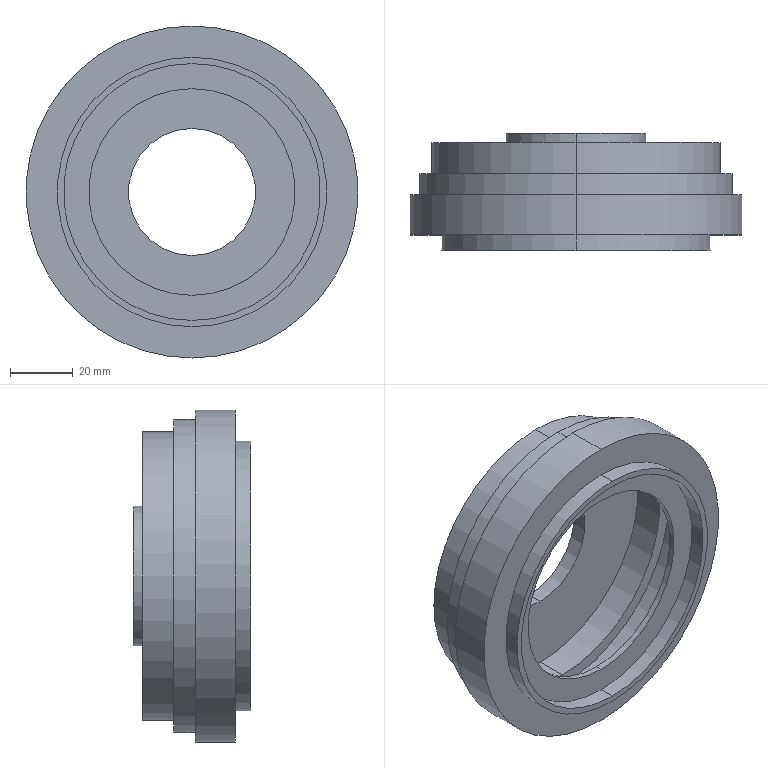Part | SolidWorks | features Revolution 1 | 1 solid | 33 faces | box 106 x 37.5 x 106 mm | volume 44844 mm3 | cylinder 22 | plane 11 | commonest cylinder face diameters 40.568 x2 44.568 x2 66 x2 82 x2 86 x2 88 x2
STEP:
#1=CARTESIAN_POINT('',(0.,136.,43.));
#2=VERTEX_POINT('',#1);
#3=CARTESIAN_POINT('',(0.,136.,-43.));
#4=VERTEX_POINT('',#3);
#5=CARTESIAN_POINT('',(0.,136.,0.));
#6=DIRECTION('',(0.,1.,0.));
#7=DIRECTION('',(0.,0.,1.));
#8=AXIS2_PLACEMENT_3D('',#5,#6,#7);
#9=CIRCLE('',#8,43.);
#10=EDGE_CURVE('',#2,#4,#9,.T.);
#11=ORIENTED_EDGE('',*,*,#10,.T.);
#12=CARTESIAN_POINT('',(0.,141.,-43.));
#13=VERTEX_POINT('',#12);
#14=CARTESIAN_POINT('',(0.,0.,-43.));
#15=DIRECTION('',(0.,1.,0.));
#16=VECTOR('',#15,1000.);
#17=LINE('',#14,#16);
#18=EDGE_CURVE('',#4,#13,#17,.T.);
#19=ORIENTED_EDGE('',*,*,#18,.T.);
#20=CARTESIAN_POINT('',(0.,141.,43.));
#21=VERTEX_POINT('',#20);
#22=CARTESIAN_POINT('',(0.,141.,0.));
#23=DIRECTION('',(0.,1.,0.));
#24=DIRECTION('',(0.,0.,1.));
#25=AXIS2_PLACEMENT_3D('',#22,#23,#24);
#26=CIRCLE('',#25,43.);
#27=EDGE_CURVE('',#21,#13,#26,.T.);
#28=ORIENTED_EDGE('',*,*,#27,.F.);
#29=CARTESIAN_POINT('',(0.,0.,43.));
#30=DIRECTION('',(0.,1.,0.));
#31=VECTOR('',#30,1000.);
#32=LINE('',#29,#31);
#33=EDGE_CURVE('',#2,#21,#32,.T.);
#34=ORIENTED_EDGE('',*,*,#33,.F.);
#35=EDGE_LOOP('',(#11,#19,#28,#34));
#36=FACE_OUTER_BOUND('',#35,.T.);
#37=CARTESIAN_POINT('',(0.,0.,0.));
#38=DIRECTION('',(0.,1.,0.));
#39=DIRECTION('',(0.,0.,1.));
#40=AXIS2_PLACEMENT_3D('',#37,#38,#39);
#41=CYLINDRICAL_SURFACE('',#40,43.);
#42=ADVANCED_FACE('',(#36),#41,.T.);
#43=CARTESIAN_POINT('',(0.,141.,53.));
#44=VERTEX_POINT('',#43);
#45=CARTESIAN_POINT('',(0.,141.,-53.));
#46=VERTEX_POINT('',#45);
#47=CARTESIAN_POINT('',(0.,141.,0.));
#48=DIRECTION('',(0.,1.,0.));
#49=DIRECTION('',(0.,0.,1.));
#50=AXIS2_PLACEMENT_3D('',#47,#48,#49);
#51=CIRCLE('',#50,53.);
#52=EDGE_CURVE('',#44,#46,#51,.T.);
#53=ORIENTED_EDGE('',*,*,#52,.T.);
#54=CARTESIAN_POINT('',(0.,153.773,-53.));
#55=VERTEX_POINT('',#54);
#56=CARTESIAN_POINT('',(0.,0.,-53.));
#57=DIRECTION('',(0.,1.,0.));
#58=VECTOR('',#57,1000.);
#59=LINE('',#56,#58);
#60=EDGE_CURVE('',#46,#55,#59,.T.);
#61=ORIENTED_EDGE('',*,*,#60,.T.);
#62=CARTESIAN_POINT('',(0.,153.773,53.));
#63=VERTEX_POINT('',#62);
#64=CARTESIAN_POINT('',(0.,153.773,0.));
#65=DIRECTION('',(0.,1.,0.));
#66=DIRECTION('',(0.,0.,1.));
#67=AXIS2_PLACEMENT_3D('',#64,#65,#66);
#68=CIRCLE('',#67,53.);
#69=EDGE_CURVE('',#63,#55,#68,.T.);
#70=ORIENTED_EDGE('',*,*,#69,.F.);
#71=CARTESIAN_POINT('',(0.,0.,53.));
#72=DIRECTION('',(0.,1.,0.));
#73=VECTOR('',#72,1000.);
#74=LINE('',#71,#73);
#75=EDGE_CURVE('',#44,#63,#74,.T.);
#76=ORIENTED_EDGE('',*,*,#75,.F.);
#77=EDGE_LOOP('',(#53,#61,#70,#76));
#78=FACE_OUTER_BOUND('',#77,.T.);
#79=CARTESIAN_POINT('',(0.,0.,0.));
#80=DIRECTION('',(0.,1.,0.));
#81=DIRECTION('',(0.,0.,1.));
#82=AXIS2_PLACEMENT_3D('',#79,#80,#81);
#83=CYLINDRICAL_SURFACE('',#82,53.);
#84=ADVANCED_FACE('',(#78),#83,.T.);
#85=CARTESIAN_POINT('',(0.,153.773,50.));
#86=VERTEX_POINT('',#85);
#87=CARTESIAN_POINT('',(0.,153.773,-50.));
#88=VERTEX_POINT('',#87);
#89=CARTESIAN_POINT('',(0.,153.773,0.));
#90=DIRECTION('',(0.,1.,0.));
#91=DIRECTION('',(0.,0.,1.));
#92=AXIS2_PLACEMENT_3D('',#89,#90,#91);
#93=CIRCLE('',#92,50.);
#94=EDGE_CURVE('',#86,#88,#93,.T.);
#95=ORIENTED_EDGE('',*,*,#94,.T.);
#96=CARTESIAN_POINT('',(0.,160.532,-50.));
#97=VERTEX_POINT('',#96);
#98=CARTESIAN_POINT('',(0.,0.,-50.));
#99=DIRECTION('',(0.,1.,0.));
#100=VECTOR('',#99,1000.);
#101=LINE('',#98,#100);
#102=EDGE_CURVE('',#88,#97,#101,.T.);
#103=ORIENTED_EDGE('',*,*,#102,.T.);
#104=CARTESIAN_POINT('',(0.,160.532,50.));
#105=VERTEX_POINT('',#104);
#106=CARTESIAN_POINT('',(0.,160.532,0.));
#107=DIRECTION('',(0.,1.,0.));
#108=DIRECTION('',(0.,0.,1.));
#109=AXIS2_PLACEMENT_3D('',#106,#107,#108);
#110=CIRCLE('',#109,50.);
#111=EDGE_CURVE('',#105,#97,#110,.T.);
#112=ORIENTED_EDGE('',*,*,#111,.F.);
#113=CARTESIAN_POINT('',(0.,0.,50.));
#114=DIRECTION('',(0.,1.,0.));
#115=VECTOR('',#114,1000.);
#116=LINE('',#113,#115);
#117=EDGE_CURVE('',#86,#105,#116,.T.);
#118=ORIENTED_EDGE('',*,*,#117,.F.);
#119=EDGE_LOOP('',(#95,#103,#112,#118));
#120=FACE_OUTER_BOUND('',#119,.T.);
#121=CARTESIAN_POINT('',(0.,0.,0.));
#122=DIRECTION('',(0.,1.,0.));
#123=DIRECTION('',(0.,0.,1.));
#124=AXIS2_PLACEMENT_3D('',#121,#122,#123);
#125=CYLINDRICAL_SURFACE('',#124,50.);
#126=ADVANCED_FACE('',(#120),#125,.T.);
#127=CARTESIAN_POINT('',(0.,160.532,46.));
#128=VERTEX_POINT('',#127);
#129=CARTESIAN_POINT('',(0.,160.532,-46.));
#130=VERTEX_POINT('',#129);
#131=CARTESIAN_POINT('',(0.,160.532,0.));
#132=DIRECTION('',(0.,1.,0.));
#133=DIRECTION('',(0.,0.,1.));
#134=AXIS2_PLACEMENT_3D('',#131,#132,#133);
#135=CIRCLE('',#134,46.);
#136=EDGE_CURVE('',#128,#130,#135,.T.);
#137=ORIENTED_EDGE('',*,*,#136,.T.);
#138=CARTESIAN_POINT('',(0.,170.5,-46.));
#139=VERTEX_POINT('',#138);
#140=CARTESIAN_POINT('',(0.,0.,-46.));
#141=DIRECTION('',(0.,1.,0.));
#142=VECTOR('',#141,1000.);
#143=LINE('',#140,#142);
#144=EDGE_CURVE('',#130,#139,#143,.T.);
#145=ORIENTED_EDGE('',*,*,#144,.T.);
#146=CARTESIAN_POINT('',(0.,170.5,46.));
#147=VERTEX_POINT('',#146);
#148=CARTESIAN_POINT('',(0.,170.5,0.));
#149=DIRECTION('',(0.,1.,0.));
#150=DIRECTION('',(0.,0.,1.));
#151=AXIS2_PLACEMENT_3D('',#148,#149,#150);
#152=CIRCLE('',#151,46.);
#153=EDGE_CURVE('',#147,#139,#152,.T.);
#154=ORIENTED_EDGE('',*,*,#153,.F.);
#155=CARTESIAN_POINT('',(0.,0.,46.));
#156=DIRECTION('',(0.,1.,0.));
#157=VECTOR('',#156,1000.);
#158=LINE('',#155,#157);
#159=EDGE_CURVE('',#128,#147,#158,.T.);
#160=ORIENTED_EDGE('',*,*,#159,.F.);
#161=EDGE_LOOP('',(#137,#145,#154,#160));
#162=FACE_OUTER_BOUND('',#161,.T.);
#163=CARTESIAN_POINT('',(0.,0.,0.));
#164=DIRECTION('',(0.,1.,0.));
#165=DIRECTION('',(0.,0.,1.));
#166=AXIS2_PLACEMENT_3D('',#163,#164,#165);
#167=CYLINDRICAL_SURFACE('',#166,46.);
#168=ADVANCED_FACE('',(#162),#167,.T.);
#169=CARTESIAN_POINT('',(0.,170.5,22.284));
#170=VERTEX_POINT('',#169);
#171=CARTESIAN_POINT('',(0.,170.5,-22.284));
#172=VERTEX_POINT('',#171);
#173=CARTESIAN_POINT('',(0.,170.5,0.));
#174=DIRECTION('',(0.,1.,0.));
#175=DIRECTION('',(0.,0.,1.));
#176=AXIS2_PLACEMENT_3D('',#173,#174,#175);
#177=CIRCLE('',#176,22.284);
#178=EDGE_CURVE('',#170,#172,#177,.T.);
#179=ORIENTED_EDGE('',*,*,#178,.T.);
#180=CARTESIAN_POINT('',(0.,173.5,-22.284));
#181=VERTEX_POINT('',#180);
#182=CARTESIAN_POINT('',(0.,0.,-22.284));
#183=DIRECTION('',(0.,1.,0.));
#184=VECTOR('',#183,1000.);
#185=LINE('',#182,#184);
#186=EDGE_CURVE('',#172,#181,#185,.T.);
#187=ORIENTED_EDGE('',*,*,#186,.T.);
#188=CARTESIAN_POINT('',(0.,173.5,22.284));
#189=VERTEX_POINT('',#188);
#190=CARTESIAN_POINT('',(0.,173.5,0.));
#191=DIRECTION('',(0.,1.,0.));
#192=DIRECTION('',(0.,0.,1.));
#193=AXIS2_PLACEMENT_3D('',#190,#191,#192);
#194=CIRCLE('',#193,22.284);
#195=EDGE_CURVE('',#189,#181,#194,.T.);
#196=ORIENTED_EDGE('',*,*,#195,.F.);
#197=CARTESIAN_POINT('',(0.,0.,22.284));
#198=DIRECTION('',(0.,1.,0.));
#199=VECTOR('',#198,1000.);
#200=LINE('',#197,#199);
#201=EDGE_CURVE('',#170,#189,#200,.T.);
#202=ORIENTED_EDGE('',*,*,#201,.F.);
#203=EDGE_LOOP('',(#179,#187,#196,#202));
#204=FACE_OUTER_BOUND('',#203,.T.);
#205=CARTESIAN_POINT('',(0.,0.,0.));
#206=DIRECTION('',(0.,1.,0.));
#207=DIRECTION('',(0.,0.,1.));
#208=AXIS2_PLACEMENT_3D('',#205,#206,#207);
#209=CYLINDRICAL_SURFACE('',#208,22.284);
#210=ADVANCED_FACE('',(#204),#209,.T.);
#211=CARTESIAN_POINT('',(0.,168.5,-20.284));
#212=VERTEX_POINT('',#211);
#213=CARTESIAN_POINT('',(0.,168.5,20.284));
#214=VERTEX_POINT('',#213);
#215=CARTESIAN_POINT('',(0.,168.5,0.));
#216=DIRECTION('',(0.,1.,0.));
#217=DIRECTION('',(0.,0.,1.));
#218=AXIS2_PLACEMENT_3D('',#215,#216,#217);
#219=CIRCLE('',#218,20.284);
#220=EDGE_CURVE('',#212,#214,#219,.T.);
#221=ORIENTED_EDGE('',*,*,#220,.F.);
#222=CARTESIAN_POINT('',(0.,173.5,-20.284));
#223=VERTEX_POINT('',#222);
#224=CARTESIAN_POINT('',(0.,0.,-20.284));
#225=DIRECTION('',(0.,1.,0.));
#226=VECTOR('',#225,1000.);
#227=LINE('',#224,#226);
#228=EDGE_CURVE('',#212,#223,#227,.T.);
#229=ORIENTED_EDGE('',*,*,#228,.T.);
#230=CARTESIAN_POINT('',(0.,173.5,20.284));
#231=VERTEX_POINT('',#230);
#232=CARTESIAN_POINT('',(0.,173.5,0.));
#233=DIRECTION('',(0.,1.,0.));
#234=DIRECTION('',(0.,0.,1.));
#235=AXIS2_PLACEMENT_3D('',#232,#233,#234);
#236=CIRCLE('',#235,20.284);
#237=EDGE_CURVE('',#223,#231,#236,.T.);
#238=ORIENTED_EDGE('',*,*,#237,.T.);
#239=CARTESIAN_POINT('',(0.,0.,20.284));
#240=DIRECTION('',(0.,1.,0.));
#241=VECTOR('',#240,1000.);
#242=LINE('',#239,#241);
#243=EDGE_CURVE('',#214,#231,#242,.T.);
#244=ORIENTED_EDGE('',*,*,#243,.F.);
#245=EDGE_LOOP('',(#221,#229,#238,#244));
#246=FACE_OUTER_BOUND('',#245,.T.);
#247=CARTESIAN_POINT('',(0.,0.,0.));
#248=DIRECTION('',(0.,1.,0.));
#249=DIRECTION('',(0.,0.,1.));
#250=AXIS2_PLACEMENT_3D('',#247,#248,#249);
#251=CYLINDRICAL_SURFACE('',#250,20.284);
#252=ADVANCED_FACE('',(#246),#251,.F.);
#253=CARTESIAN_POINT('',(0.,158.532,-44.));
#254=VERTEX_POINT('',#253);
#255=CARTESIAN_POINT('',(0.,158.532,44.));
#256=VERTEX_POINT('',#255);
#257=CARTESIAN_POINT('',(0.,158.532,0.));
#258=DIRECTION('',(0.,1.,0.));
#259=DIRECTION('',(0.,0.,1.));
#260=AXIS2_PLACEMENT_3D('',#257,#258,#259);
#261=CIRCLE('',#260,44.);
#262=EDGE_CURVE('',#254,#256,#261,.T.);
#263=ORIENTED_EDGE('',*,*,#262,.F.);
#264=CARTESIAN_POINT('',(0.,168.5,-44.));
#265=VERTEX_POINT('',#264);
#266=CARTESIAN_POINT('',(0.,0.,-44.));
#267=DIRECTION('',(0.,1.,0.));
#268=VECTOR('',#267,1000.);
#269=LINE('',#266,#268);
#270=EDGE_CURVE('',#254,#265,#269,.T.);
#271=ORIENTED_EDGE('',*,*,#270,.T.);
#272=CARTESIAN_POINT('',(0.,168.5,44.));
#273=VERTEX_POINT('',#272);
#274=CARTESIAN_POINT('',(0.,168.5,0.));
#275=DIRECTION('',(0.,1.,0.));
#276=DIRECTION('',(0.,0.,1.));
#277=AXIS2_PLACEMENT_3D('',#274,#275,#276);
#278=CIRCLE('',#277,44.);
#279=EDGE_CURVE('',#265,#273,#278,.T.);
#280=ORIENTED_EDGE('',*,*,#279,.T.);
#281=CARTESIAN_POINT('',(0.,0.,44.));
#282=DIRECTION('',(0.,1.,0.));
#283=VECTOR('',#282,1000.);
#284=LINE('',#281,#283);
#285=EDGE_CURVE('',#256,#273,#284,.T.);
#286=ORIENTED_EDGE('',*,*,#285,.F.);
#287=EDGE_LOOP('',(#263,#271,#280,#286));
#288=FACE_OUTER_BOUND('',#287,.T.);
#289=CARTESIAN_POINT('',(0.,0.,0.));
#290=DIRECTION('',(0.,1.,0.));
#291=DIRECTION('',(0.,0.,1.));
#292=AXIS2_PLACEMENT_3D('',#289,#290,#291);
#293=CYLINDRICAL_SURFACE('',#292,44.);
#294=ADVANCED_FACE('',(#288),#293,.F.);
#295=CARTESIAN_POINT('',(0.,151.773,-48.));
#296=VERTEX_POINT('',#295);
#297=CARTESIAN_POINT('',(0.,151.773,48.));
#298=VERTEX_POINT('',#297);
#299=CARTESIAN_POINT('',(0.,151.773,0.));
#300=DIRECTION('',(0.,1.,0.));
#301=DIRECTION('',(0.,0.,1.));
#302=AXIS2_PLACEMENT_3D('',#299,#300,#301);
#303=CIRCLE('',#302,48.);
#304=EDGE_CURVE('',#296,#298,#303,.T.);
#305=ORIENTED_EDGE('',*,*,#304,.F.);
#306=CARTESIAN_POINT('',(0.,158.532,-48.));
#307=VERTEX_POINT('',#306);
#308=CARTESIAN_POINT('',(0.,0.,-48.));
#309=DIRECTION('',(0.,1.,0.));
#310=VECTOR('',#309,1000.);
#311=LINE('',#308,#310);
#312=EDGE_CURVE('',#296,#307,#311,.T.);
#313=ORIENTED_EDGE('',*,*,#312,.T.);
#314=CARTESIAN_POINT('',(0.,158.532,48.));
#315=VERTEX_POINT('',#314);
#316=CARTESIAN_POINT('',(0.,158.532,0.));
#317=DIRECTION('',(0.,1.,0.));
#318=DIRECTION('',(0.,0.,1.));
#319=AXIS2_PLACEMENT_3D('',#316,#317,#318);
#320=CIRCLE('',#319,48.);
#321=EDGE_CURVE('',#307,#315,#320,.T.);
#322=ORIENTED_EDGE('',*,*,#321,.T.);
#323=CARTESIAN_POINT('',(0.,0.,48.));
#324=DIRECTION('',(0.,1.,0.));
#325=VECTOR('',#324,1000.);
#326=LINE('',#323,#325);
#327=EDGE_CURVE('',#298,#315,#326,.T.);
#328=ORIENTED_EDGE('',*,*,#327,.F.);
#329=EDGE_LOOP('',(#305,#313,#322,#328));
#330=FACE_OUTER_BOUND('',#329,.T.);
#331=CARTESIAN_POINT('',(0.,0.,0.));
#332=DIRECTION('',(0.,1.,0.));
#333=DIRECTION('',(0.,0.,1.));
#334=AXIS2_PLACEMENT_3D('',#331,#332,#333);
#335=CYLINDRICAL_SURFACE('',#334,48.);
#336=ADVANCED_FACE('',(#330),#335,.F.);
#337=CARTESIAN_POINT('',(0.,143.,-51.));
#338=VERTEX_POINT('',#337);
#339=CARTESIAN_POINT('',(0.,143.,51.));
#340=VERTEX_POINT('',#339);
#341=CARTESIAN_POINT('',(0.,143.,0.));
#342=DIRECTION('',(0.,1.,0.));
#343=DIRECTION('',(0.,0.,1.));
#344=AXIS2_PLACEMENT_3D('',#341,#342,#343);
#345=CIRCLE('',#344,51.);
#346=EDGE_CURVE('',#338,#340,#345,.T.);
#347=ORIENTED_EDGE('',*,*,#346,.F.);
#348=CARTESIAN_POINT('',(0.,151.773,-51.));
#349=VERTEX_POINT('',#348);
#350=CARTESIAN_POINT('',(0.,0.,-51.));
#351=DIRECTION('',(0.,1.,0.));
#352=VECTOR('',#351,1000.);
#353=LINE('',#350,#352);
#354=EDGE_CURVE('',#338,#349,#353,.T.);
#355=ORIENTED_EDGE('',*,*,#354,.T.);
#356=CARTESIAN_POINT('',(0.,151.773,51.));
#357=VERTEX_POINT('',#356);
#358=CARTESIAN_POINT('',(0.,151.773,0.));
#359=DIRECTION('',(0.,1.,0.));
#360=DIRECTION('',(0.,0.,1.));
#361=AXIS2_PLACEMENT_3D('',#358,#359,#360);
#362=CIRCLE('',#361,51.);
#363=EDGE_CURVE('',#349,#357,#362,.T.);
#364=ORIENTED_EDGE('',*,*,#363,.T.);
#365=CARTESIAN_POINT('',(0.,0.,51.));
#366=DIRECTION('',(0.,1.,0.));
#367=VECTOR('',#366,1000.);
#368=LINE('',#365,#367);
#369=EDGE_CURVE('',#340,#357,#368,.T.);
#370=ORIENTED_EDGE('',*,*,#369,.F.);
#371=EDGE_LOOP('',(#347,#355,#364,#370));
#372=FACE_OUTER_BOUND('',#371,.T.);
#373=CARTESIAN_POINT('',(0.,0.,0.));
#374=DIRECTION('',(0.,1.,0.));
#375=DIRECTION('',(0.,0.,1.));
#376=AXIS2_PLACEMENT_3D('',#373,#374,#375);
#377=CYLINDRICAL_SURFACE('',#376,51.);
#378=ADVANCED_FACE('',(#372),#377,.F.);
#379=CARTESIAN_POINT('',(0.,141.,-33.));
#380=VERTEX_POINT('',#379);
#381=CARTESIAN_POINT('',(0.,141.,33.));
#382=VERTEX_POINT('',#381);
#383=CARTESIAN_POINT('',(0.,141.,0.));
#384=DIRECTION('',(0.,1.,0.));
#385=DIRECTION('',(0.,0.,1.));
#386=AXIS2_PLACEMENT_3D('',#383,#384,#385);
#387=CIRCLE('',#386,33.);
#388=EDGE_CURVE('',#380,#382,#387,.T.);
#389=ORIENTED_EDGE('',*,*,#388,.F.);
#390=CARTESIAN_POINT('',(0.,143.,-33.));
#391=VERTEX_POINT('',#390);
#392=CARTESIAN_POINT('',(0.,0.,-33.));
#393=DIRECTION('',(0.,1.,0.));
#394=VECTOR('',#393,1000.);
#395=LINE('',#392,#394);
#396=EDGE_CURVE('',#380,#391,#395,.T.);
#397=ORIENTED_EDGE('',*,*,#396,.T.);
#398=CARTESIAN_POINT('',(0.,143.,33.));
#399=VERTEX_POINT('',#398);
#400=CARTESIAN_POINT('',(0.,143.,0.));
#401=DIRECTION('',(0.,1.,0.));
#402=DIRECTION('',(0.,0.,1.));
#403=AXIS2_PLACEMENT_3D('',#400,#401,#402);
#404=CIRCLE('',#403,33.);
#405=EDGE_CURVE('',#391,#399,#404,.T.);
#406=ORIENTED_EDGE('',*,*,#405,.T.);
#407=CARTESIAN_POINT('',(0.,0.,33.));
#408=DIRECTION('',(0.,1.,0.));
#409=VECTOR('',#408,1000.);
#410=LINE('',#407,#409);
#411=EDGE_CURVE('',#382,#399,#410,.T.);
#412=ORIENTED_EDGE('',*,*,#411,.F.);
#413=EDGE_LOOP('',(#389,#397,#406,#412));
#414=FACE_OUTER_BOUND('',#413,.T.);
#415=CARTESIAN_POINT('',(0.,0.,0.));
#416=DIRECTION('',(0.,1.,0.));
#417=DIRECTION('',(0.,0.,1.));
#418=AXIS2_PLACEMENT_3D('',#415,#416,#417);
#419=CYLINDRICAL_SURFACE('',#418,33.);
#420=ADVANCED_FACE('',(#414),#419,.F.);
#421=CARTESIAN_POINT('',(0.,136.,-41.));
#422=VERTEX_POINT('',#421);
#423=CARTESIAN_POINT('',(0.,136.,41.));
#424=VERTEX_POINT('',#423);
#425=CARTESIAN_POINT('',(0.,136.,0.));
#426=DIRECTION('',(0.,1.,0.));
#427=DIRECTION('',(0.,0.,1.));
#428=AXIS2_PLACEMENT_3D('',#425,#426,#427);
#429=CIRCLE('',#428,41.);
#430=EDGE_CURVE('',#422,#424,#429,.T.);
#431=ORIENTED_EDGE('',*,*,#430,.F.);
#432=CARTESIAN_POINT('',(0.,141.,-41.));
#433=VERTEX_POINT('',#432);
#434=CARTESIAN_POINT('',(0.,0.,-41.));
#435=DIRECTION('',(0.,1.,0.));
#436=VECTOR('',#435,1000.);
#437=LINE('',#434,#436);
#438=EDGE_CURVE('',#422,#433,#437,.T.);
#439=ORIENTED_EDGE('',*,*,#438,.T.);
#440=CARTESIAN_POINT('',(0.,141.,41.));
#441=VERTEX_POINT('',#440);
#442=CARTESIAN_POINT('',(0.,141.,0.));
#443=DIRECTION('',(0.,1.,0.));
#444=DIRECTION('',(0.,0.,1.));
#445=AXIS2_PLACEMENT_3D('',#442,#443,#444);
#446=CIRCLE('',#445,41.);
#447=EDGE_CURVE('',#433,#441,#446,.T.);
#448=ORIENTED_EDGE('',*,*,#447,.T.);
#449=CARTESIAN_POINT('',(0.,0.,41.));
#450=DIRECTION('',(0.,1.,0.));
#451=VECTOR('',#450,1000.);
#452=LINE('',#449,#451);
#453=EDGE_CURVE('',#424,#441,#452,.T.);
#454=ORIENTED_EDGE('',*,*,#453,.F.);
#455=EDGE_LOOP('',(#431,#439,#448,#454));
#456=FACE_OUTER_BOUND('',#455,.T.);
#457=CARTESIAN_POINT('',(0.,0.,0.));
#458=DIRECTION('',(0.,1.,0.));
#459=DIRECTION('',(0.,0.,1.));
#460=AXIS2_PLACEMENT_3D('',#457,#458,#459);
#461=CYLINDRICAL_SURFACE('',#460,41.);
#462=ADVANCED_FACE('',(#456),#461,.F.);
#463=ORIENTED_EDGE('',*,*,#10,.F.);
#464=CARTESIAN_POINT('',(0.,136.,0.));
#465=DIRECTION('',(0.,1.,0.));
#466=DIRECTION('',(0.,0.,1.));
#467=AXIS2_PLACEMENT_3D('',#464,#465,#466);
#468=CIRCLE('',#467,43.);
#469=EDGE_CURVE('',#4,#2,#468,.T.);
#470=ORIENTED_EDGE('',*,*,#469,.F.);
#471=EDGE_LOOP('',(#463,#470));
#472=FACE_OUTER_BOUND('',#471,.T.);
#473=CARTESIAN_POINT('',(0.,136.,0.));
#474=DIRECTION('',(0.,1.,0.));
#475=DIRECTION('',(0.,0.,1.));
#476=AXIS2_PLACEMENT_3D('',#473,#474,#475);
#477=CIRCLE('',#476,41.);
#478=EDGE_CURVE('',#424,#422,#477,.T.);
#479=ORIENTED_EDGE('',*,*,#478,.T.);
#480=ORIENTED_EDGE('',*,*,#430,.T.);
#481=EDGE_LOOP('',(#479,#480));
#482=FACE_BOUND('',#481,.T.);
#483=CARTESIAN_POINT('',(43.,136.,0.));
#484=DIRECTION('',(0.,1.,0.));
#485=DIRECTION('',(0.,0.,1.));
#486=AXIS2_PLACEMENT_3D('',#483,#484,#485);
#487=PLANE('',#486);
#488=ADVANCED_FACE('',(#472,#482),#487,.F.);
#489=ORIENTED_EDGE('',*,*,#438,.F.);
#490=ORIENTED_EDGE('',*,*,#478,.F.);
#491=ORIENTED_EDGE('',*,*,#453,.T.);
#492=CARTESIAN_POINT('',(0.,141.,0.));
#493=DIRECTION('',(0.,1.,0.));
#494=DIRECTION('',(0.,0.,1.));
#495=AXIS2_PLACEMENT_3D('',#492,#493,#494);
#496=CIRCLE('',#495,41.);
#497=EDGE_CURVE('',#441,#433,#496,.T.);
#498=ORIENTED_EDGE('',*,*,#497,.T.);
#499=EDGE_LOOP('',(#489,#490,#491,#498));
#500=FACE_OUTER_BOUND('',#499,.T.);
#501=CARTESIAN_POINT('',(0.,0.,0.));
#502=DIRECTION('',(0.,1.,0.));
#503=DIRECTION('',(0.,0.,1.));
#504=AXIS2_PLACEMENT_3D('',#501,#502,#503);
#505=CYLINDRICAL_SURFACE('',#504,41.);
#506=ADVANCED_FACE('',(#500),#505,.F.);
#507=ORIENTED_EDGE('',*,*,#497,.F.);
#508=ORIENTED_EDGE('',*,*,#447,.F.);
#509=EDGE_LOOP('',(#507,#508));
#510=FACE_OUTER_BOUND('',#509,.T.);
#511=CARTESIAN_POINT('',(0.,141.,0.));
#512=DIRECTION('',(0.,1.,0.));
#513=DIRECTION('',(0.,0.,1.));
#514=AXIS2_PLACEMENT_3D('',#511,#512,#513);
#515=CIRCLE('',#514,33.);
#516=EDGE_CURVE('',#382,#380,#515,.T.);
#517=ORIENTED_EDGE('',*,*,#516,.T.);
#518=ORIENTED_EDGE('',*,*,#388,.T.);
#519=EDGE_LOOP('',(#517,#518));
#520=FACE_BOUND('',#519,.T.);
#521=CARTESIAN_POINT('',(41.,141.,0.));
#522=DIRECTION('',(0.,1.,0.));
#523=DIRECTION('',(0.,0.,1.));
#524=AXIS2_PLACEMENT_3D('',#521,#522,#523);
#525=PLANE('',#524);
#526=ADVANCED_FACE('',(#510,#520),#525,.F.);
#527=ORIENTED_EDGE('',*,*,#396,.F.);
#528=ORIENTED_EDGE('',*,*,#516,.F.);
#529=ORIENTED_EDGE('',*,*,#411,.T.);
#530=CARTESIAN_POINT('',(0.,143.,0.));
#531=DIRECTION('',(0.,1.,0.));
#532=DIRECTION('',(0.,0.,1.));
#533=AXIS2_PLACEMENT_3D('',#530,#531,#532);
#534=CIRCLE('',#533,33.);
#535=EDGE_CURVE('',#399,#391,#534,.T.);
#536=ORIENTED_EDGE('',*,*,#535,.T.);
#537=EDGE_LOOP('',(#527,#528,#529,#536));
#538=FACE_OUTER_BOUND('',#537,.T.);
#539=CARTESIAN_POINT('',(0.,0.,0.));
#540=DIRECTION('',(0.,1.,0.));
#541=DIRECTION('',(0.,0.,1.));
#542=AXIS2_PLACEMENT_3D('',#539,#540,#541);
#543=CYLINDRICAL_SURFACE('',#542,33.);
#544=ADVANCED_FACE('',(#538),#543,.F.);
#545=ORIENTED_EDGE('',*,*,#535,.F.);
#546=ORIENTED_EDGE('',*,*,#405,.F.);
#547=EDGE_LOOP('',(#545,#546));
#548=FACE_BOUND('',#547,.T.);
#549=CARTESIAN_POINT('',(0.,143.,0.));
#550=DIRECTION('',(0.,1.,0.));
#551=DIRECTION('',(0.,0.,1.));
#552=AXIS2_PLACEMENT_3D('',#549,#550,#551);
#553=CIRCLE('',#552,51.);
#554=EDGE_CURVE('',#340,#338,#553,.T.);
#555=ORIENTED_EDGE('',*,*,#554,.T.);
#556=ORIENTED_EDGE('',*,*,#346,.T.);
#557=EDGE_LOOP('',(#555,#556));
#558=FACE_OUTER_BOUND('',#557,.T.);
#559=CARTESIAN_POINT('',(41.,143.,0.));
#560=DIRECTION('',(0.,-1.,0.));
#561=DIRECTION('',(0.,0.,-1.));
#562=AXIS2_PLACEMENT_3D('',#559,#560,#561);
#563=PLANE('',#562);
#564=ADVANCED_FACE('',(#548,#558),#563,.F.);
#565=ORIENTED_EDGE('',*,*,#354,.F.);
#566=ORIENTED_EDGE('',*,*,#554,.F.);
#567=ORIENTED_EDGE('',*,*,#369,.T.);
#568=CARTESIAN_POINT('',(0.,151.773,0.));
#569=DIRECTION('',(0.,1.,0.));
#570=DIRECTION('',(0.,0.,1.));
#571=AXIS2_PLACEMENT_3D('',#568,#569,#570);
#572=CIRCLE('',#571,51.);
#573=EDGE_CURVE('',#357,#349,#572,.T.);
#574=ORIENTED_EDGE('',*,*,#573,.T.);
#575=EDGE_LOOP('',(#565,#566,#567,#574));
#576=FACE_OUTER_BOUND('',#575,.T.);
#577=CARTESIAN_POINT('',(0.,0.,0.));
#578=DIRECTION('',(0.,1.,0.));
#579=DIRECTION('',(0.,0.,1.));
#580=AXIS2_PLACEMENT_3D('',#577,#578,#579);
#581=CYLINDRICAL_SURFACE('',#580,51.);
#582=ADVANCED_FACE('',(#576),#581,.F.);
#583=ORIENTED_EDGE('',*,*,#573,.F.);
#584=ORIENTED_EDGE('',*,*,#363,.F.);
#585=EDGE_LOOP('',(#583,#584));
#586=FACE_OUTER_BOUND('',#585,.T.);
#587=CARTESIAN_POINT('',(0.,151.773,0.));
#588=DIRECTION('',(0.,1.,0.));
#589=DIRECTION('',(0.,0.,1.));
#590=AXIS2_PLACEMENT_3D('',#587,#588,#589);
#591=CIRCLE('',#590,48.);
#592=EDGE_CURVE('',#298,#296,#591,.T.);
#593=ORIENTED_EDGE('',*,*,#592,.T.);
#594=ORIENTED_EDGE('',*,*,#304,.T.);
#595=EDGE_LOOP('',(#593,#594));
#596=FACE_BOUND('',#595,.T.);
#597=CARTESIAN_POINT('',(51.,151.773,0.));
#598=DIRECTION('',(0.,1.,0.));
#599=DIRECTION('',(0.,0.,1.));
#600=AXIS2_PLACEMENT_3D('',#597,#598,#599);
#601=PLANE('',#600);
#602=ADVANCED_FACE('',(#586,#596),#601,.F.);
#603=ORIENTED_EDGE('',*,*,#312,.F.);
#604=ORIENTED_EDGE('',*,*,#592,.F.);
#605=ORIENTED_EDGE('',*,*,#327,.T.);
#606=CARTESIAN_POINT('',(0.,158.532,0.));
#607=DIRECTION('',(0.,1.,0.));
#608=DIRECTION('',(0.,0.,1.));
#609=AXIS2_PLACEMENT_3D('',#606,#607,#608);
#610=CIRCLE('',#609,48.);
#611=EDGE_CURVE('',#315,#307,#610,.T.);
#612=ORIENTED_EDGE('',*,*,#611,.T.);
#613=EDGE_LOOP('',(#603,#604,#605,#612));
#614=FACE_OUTER_BOUND('',#613,.T.);
#615=CARTESIAN_POINT('',(0.,0.,0.));
#616=DIRECTION('',(0.,1.,0.));
#617=DIRECTION('',(0.,0.,1.));
#618=AXIS2_PLACEMENT_3D('',#615,#616,#617);
#619=CYLINDRICAL_SURFACE('',#618,48.);
#620=ADVANCED_FACE('',(#614),#619,.F.);
#621=ORIENTED_EDGE('',*,*,#611,.F.);
#622=ORIENTED_EDGE('',*,*,#321,.F.);
#623=EDGE_LOOP('',(#621,#622));
#624=FACE_OUTER_BOUND('',#623,.T.);
#625=CARTESIAN_POINT('',(0.,158.532,0.));
#626=DIRECTION('',(0.,1.,0.));
#627=DIRECTION('',(0.,0.,1.));
#628=AXIS2_PLACEMENT_3D('',#625,#626,#627);
#629=CIRCLE('',#628,44.);
#630=EDGE_CURVE('',#256,#254,#629,.T.);
#631=ORIENTED_EDGE('',*,*,#630,.T.);
#632=ORIENTED_EDGE('',*,*,#262,.T.);
#633=EDGE_LOOP('',(#631,#632));
#634=FACE_BOUND('',#633,.T.);
#635=CARTESIAN_POINT('',(48.,158.532,0.));
#636=DIRECTION('',(0.,1.,0.));
#637=DIRECTION('',(0.,0.,1.));
#638=AXIS2_PLACEMENT_3D('',#635,#636,#637);
#639=PLANE('',#638);
#640=ADVANCED_FACE('',(#624,#634),#639,.F.);
#641=ORIENTED_EDGE('',*,*,#270,.F.);
#642=ORIENTED_EDGE('',*,*,#630,.F.);
#643=ORIENTED_EDGE('',*,*,#285,.T.);
#644=CARTESIAN_POINT('',(0.,168.5,0.));
#645=DIRECTION('',(0.,1.,0.));
#646=DIRECTION('',(0.,0.,1.));
#647=AXIS2_PLACEMENT_3D('',#644,#645,#646);
#648=CIRCLE('',#647,44.);
#649=EDGE_CURVE('',#273,#265,#648,.T.);
#650=ORIENTED_EDGE('',*,*,#649,.T.);
#651=EDGE_LOOP('',(#641,#642,#643,#650));
#652=FACE_OUTER_BOUND('',#651,.T.);
#653=CARTESIAN_POINT('',(0.,0.,0.));
#654=DIRECTION('',(0.,1.,0.));
#655=DIRECTION('',(0.,0.,1.));
#656=AXIS2_PLACEMENT_3D('',#653,#654,#655);
#657=CYLINDRICAL_SURFACE('',#656,44.);
#658=ADVANCED_FACE('',(#652),#657,.F.);
#659=ORIENTED_EDGE('',*,*,#649,.F.);
#660=ORIENTED_EDGE('',*,*,#279,.F.);
#661=EDGE_LOOP('',(#659,#660));
#662=FACE_OUTER_BOUND('',#661,.T.);
#663=CARTESIAN_POINT('',(0.,168.5,0.));
#664=DIRECTION('',(0.,1.,0.));
#665=DIRECTION('',(0.,0.,1.));
#666=AXIS2_PLACEMENT_3D('',#663,#664,#665);
#667=CIRCLE('',#666,20.284);
#668=EDGE_CURVE('',#214,#212,#667,.T.);
#669=ORIENTED_EDGE('',*,*,#668,.T.);
#670=ORIENTED_EDGE('',*,*,#220,.T.);
#671=EDGE_LOOP('',(#669,#670));
#672=FACE_BOUND('',#671,.T.);
#673=CARTESIAN_POINT('',(44.,168.5,0.));
#674=DIRECTION('',(0.,1.,0.));
#675=DIRECTION('',(0.,0.,1.));
#676=AXIS2_PLACEMENT_3D('',#673,#674,#675);
#677=PLANE('',#676);
#678=ADVANCED_FACE('',(#662,#672),#677,.F.);
#679=ORIENTED_EDGE('',*,*,#228,.F.);
#680=ORIENTED_EDGE('',*,*,#668,.F.);
#681=ORIENTED_EDGE('',*,*,#243,.T.);
#682=CARTESIAN_POINT('',(0.,173.5,0.));
#683=DIRECTION('',(0.,1.,0.));
#684=DIRECTION('',(0.,0.,1.));
#685=AXIS2_PLACEMENT_3D('',#682,#683,#684);
#686=CIRCLE('',#685,20.284);
#687=EDGE_CURVE('',#231,#223,#686,.T.);
#688=ORIENTED_EDGE('',*,*,#687,.T.);
#689=EDGE_LOOP('',(#679,#680,#681,#688));
#690=FACE_OUTER_BOUND('',#689,.T.);
#691=CARTESIAN_POINT('',(0.,0.,0.));
#692=DIRECTION('',(0.,1.,0.));
#693=DIRECTION('',(0.,0.,1.));
#694=AXIS2_PLACEMENT_3D('',#691,#692,#693);
#695=CYLINDRICAL_SURFACE('',#694,20.284);
#696=ADVANCED_FACE('',(#690),#695,.F.);
#697=ORIENTED_EDGE('',*,*,#687,.F.);
#698=ORIENTED_EDGE('',*,*,#237,.F.);
#699=EDGE_LOOP('',(#697,#698));
#700=FACE_BOUND('',#699,.T.);
#701=ORIENTED_EDGE('',*,*,#195,.T.);
#702=CARTESIAN_POINT('',(0.,173.5,0.));
#703=DIRECTION('',(0.,1.,0.));
#704=DIRECTION('',(0.,0.,1.));
#705=AXIS2_PLACEMENT_3D('',#702,#703,#704);
#706=CIRCLE('',#705,22.284);
#707=EDGE_CURVE('',#181,#189,#706,.T.);
#708=ORIENTED_EDGE('',*,*,#707,.T.);
#709=EDGE_LOOP('',(#701,#708));
#710=FACE_OUTER_BOUND('',#709,.T.);
#711=CARTESIAN_POINT('',(22.284,173.5,0.));
#712=DIRECTION('',(0.,-1.,0.));
#713=DIRECTION('',(0.,0.,-1.));
#714=AXIS2_PLACEMENT_3D('',#711,#712,#713);
#715=PLANE('',#714);
#716=ADVANCED_FACE('',(#700,#710),#715,.F.);
#717=ORIENTED_EDGE('',*,*,#186,.F.);
#718=CARTESIAN_POINT('',(0.,170.5,0.));
#719=DIRECTION('',(0.,1.,0.));
#720=DIRECTION('',(0.,0.,1.));
#721=AXIS2_PLACEMENT_3D('',#718,#719,#720);
#722=CIRCLE('',#721,22.284);
#723=EDGE_CURVE('',#172,#170,#722,.T.);
#724=ORIENTED_EDGE('',*,*,#723,.T.);
#725=ORIENTED_EDGE('',*,*,#201,.T.);
#726=ORIENTED_EDGE('',*,*,#707,.F.);
#727=EDGE_LOOP('',(#717,#724,#725,#726));
#728=FACE_OUTER_BOUND('',#727,.T.);
#729=CARTESIAN_POINT('',(0.,0.,0.));
#730=DIRECTION('',(0.,1.,0.));
#731=DIRECTION('',(0.,0.,1.));
#732=AXIS2_PLACEMENT_3D('',#729,#730,#731);
#733=CYLINDRICAL_SURFACE('',#732,22.284);
#734=ADVANCED_FACE('',(#728),#733,.T.);
#735=ORIENTED_EDGE('',*,*,#178,.F.);
#736=ORIENTED_EDGE('',*,*,#723,.F.);
#737=EDGE_LOOP('',(#735,#736));
#738=FACE_BOUND('',#737,.T.);
#739=ORIENTED_EDGE('',*,*,#153,.T.);
#740=CARTESIAN_POINT('',(0.,170.5,0.));
#741=DIRECTION('',(0.,1.,0.));
#742=DIRECTION('',(0.,0.,1.));
#743=AXIS2_PLACEMENT_3D('',#740,#741,#742);
#744=CIRCLE('',#743,46.);
#745=EDGE_CURVE('',#139,#147,#744,.T.);
#746=ORIENTED_EDGE('',*,*,#745,.T.);
#747=EDGE_LOOP('',(#739,#746));
#748=FACE_OUTER_BOUND('',#747,.T.);
#749=CARTESIAN_POINT('',(46.,170.5,0.));
#750=DIRECTION('',(0.,-1.,0.));
#751=DIRECTION('',(0.,0.,-1.));
#752=AXIS2_PLACEMENT_3D('',#749,#750,#751);
#753=PLANE('',#752);
#754=ADVANCED_FACE('',(#738,#748),#753,.F.);
#755=ORIENTED_EDGE('',*,*,#144,.F.);
#756=CARTESIAN_POINT('',(0.,160.532,0.));
#757=DIRECTION('',(0.,1.,0.));
#758=DIRECTION('',(0.,0.,1.));
#759=AXIS2_PLACEMENT_3D('',#756,#757,#758);
#760=CIRCLE('',#759,46.);
#761=EDGE_CURVE('',#130,#128,#760,.T.);
#762=ORIENTED_EDGE('',*,*,#761,.T.);
#763=ORIENTED_EDGE('',*,*,#159,.T.);
#764=ORIENTED_EDGE('',*,*,#745,.F.);
#765=EDGE_LOOP('',(#755,#762,#763,#764));
#766=FACE_OUTER_BOUND('',#765,.T.);
#767=CARTESIAN_POINT('',(0.,0.,0.));
#768=DIRECTION('',(0.,1.,0.));
#769=DIRECTION('',(0.,0.,1.));
#770=AXIS2_PLACEMENT_3D('',#767,#768,#769);
#771=CYLINDRICAL_SURFACE('',#770,46.);
#772=ADVANCED_FACE('',(#766),#771,.T.);
#773=ORIENTED_EDGE('',*,*,#136,.F.);
#774=ORIENTED_EDGE('',*,*,#761,.F.);
#775=EDGE_LOOP('',(#773,#774));
#776=FACE_BOUND('',#775,.T.);
#777=ORIENTED_EDGE('',*,*,#111,.T.);
#778=CARTESIAN_POINT('',(0.,160.532,0.));
#779=DIRECTION('',(0.,1.,0.));
#780=DIRECTION('',(0.,0.,1.));
#781=AXIS2_PLACEMENT_3D('',#778,#779,#780);
#782=CIRCLE('',#781,50.);
#783=EDGE_CURVE('',#97,#105,#782,.T.);
#784=ORIENTED_EDGE('',*,*,#783,.T.);
#785=EDGE_LOOP('',(#777,#784));
#786=FACE_OUTER_BOUND('',#785,.T.);
#787=CARTESIAN_POINT('',(50.,160.532,0.));
#788=DIRECTION('',(0.,-1.,0.));
#789=DIRECTION('',(0.,0.,-1.));
#790=AXIS2_PLACEMENT_3D('',#787,#788,#789);
#791=PLANE('',#790);
#792=ADVANCED_FACE('',(#776,#786),#791,.F.);
#793=ORIENTED_EDGE('',*,*,#102,.F.);
#794=CARTESIAN_POINT('',(0.,153.773,0.));
#795=DIRECTION('',(0.,1.,0.));
#796=DIRECTION('',(0.,0.,1.));
#797=AXIS2_PLACEMENT_3D('',#794,#795,#796);
#798=CIRCLE('',#797,50.);
#799=EDGE_CURVE('',#88,#86,#798,.T.);
#800=ORIENTED_EDGE('',*,*,#799,.T.);
#801=ORIENTED_EDGE('',*,*,#117,.T.);
#802=ORIENTED_EDGE('',*,*,#783,.F.);
#803=EDGE_LOOP('',(#793,#800,#801,#802));
#804=FACE_OUTER_BOUND('',#803,.T.);
#805=CARTESIAN_POINT('',(0.,0.,0.));
#806=DIRECTION('',(0.,1.,0.));
#807=DIRECTION('',(0.,0.,1.));
#808=AXIS2_PLACEMENT_3D('',#805,#806,#807);
#809=CYLINDRICAL_SURFACE('',#808,50.);
#810=ADVANCED_FACE('',(#804),#809,.T.);
#811=ORIENTED_EDGE('',*,*,#94,.F.);
#812=ORIENTED_EDGE('',*,*,#799,.F.);
#813=EDGE_LOOP('',(#811,#812));
#814=FACE_BOUND('',#813,.T.);
#815=ORIENTED_EDGE('',*,*,#69,.T.);
#816=CARTESIAN_POINT('',(0.,153.773,0.));
#817=DIRECTION('',(0.,1.,0.));
#818=DIRECTION('',(0.,0.,1.));
#819=AXIS2_PLACEMENT_3D('',#816,#817,#818);
#820=CIRCLE('',#819,53.);
#821=EDGE_CURVE('',#55,#63,#820,.T.);
#822=ORIENTED_EDGE('',*,*,#821,.T.);
#823=EDGE_LOOP('',(#815,#822));
#824=FACE_OUTER_BOUND('',#823,.T.);
#825=CARTESIAN_POINT('',(53.,153.773,0.));
#826=DIRECTION('',(0.,-1.,0.));
#827=DIRECTION('',(0.,0.,-1.));
#828=AXIS2_PLACEMENT_3D('',#825,#826,#827);
#829=PLANE('',#828);
#830=ADVANCED_FACE('',(#814,#824),#829,.F.);
#831=ORIENTED_EDGE('',*,*,#60,.F.);
#832=CARTESIAN_POINT('',(0.,141.,0.));
#833=DIRECTION('',(0.,1.,0.));
#834=DIRECTION('',(0.,0.,1.));
#835=AXIS2_PLACEMENT_3D('',#832,#833,#834);
#836=CIRCLE('',#835,53.);
#837=EDGE_CURVE('',#46,#44,#836,.T.);
#838=ORIENTED_EDGE('',*,*,#837,.T.);
#839=ORIENTED_EDGE('',*,*,#75,.T.);
#840=ORIENTED_EDGE('',*,*,#821,.F.);
#841=EDGE_LOOP('',(#831,#838,#839,#840));
#842=FACE_OUTER_BOUND('',#841,.T.);
#843=CARTESIAN_POINT('',(0.,0.,0.));
#844=DIRECTION('',(0.,1.,0.));
#845=DIRECTION('',(0.,0.,1.));
#846=AXIS2_PLACEMENT_3D('',#843,#844,#845);
#847=CYLINDRICAL_SURFACE('',#846,53.);
#848=ADVANCED_FACE('',(#842),#847,.T.);
#849=ORIENTED_EDGE('',*,*,#52,.F.);
#850=ORIENTED_EDGE('',*,*,#837,.F.);
#851=EDGE_LOOP('',(#849,#850));
#852=FACE_OUTER_BOUND('',#851,.T.);
#853=ORIENTED_EDGE('',*,*,#27,.T.);
#854=CARTESIAN_POINT('',(0.,141.,0.));
#855=DIRECTION('',(0.,1.,0.));
#856=DIRECTION('',(0.,0.,1.));
#857=AXIS2_PLACEMENT_3D('',#854,#855,#856);
#858=CIRCLE('',#857,43.);
#859=EDGE_CURVE('',#13,#21,#858,.T.);
#860=ORIENTED_EDGE('',*,*,#859,.T.);
#861=EDGE_LOOP('',(#853,#860));
#862=FACE_BOUND('',#861,.T.);
#863=CARTESIAN_POINT('',(43.,141.,0.));
#864=DIRECTION('',(0.,1.,0.));
#865=DIRECTION('',(0.,0.,1.));
#866=AXIS2_PLACEMENT_3D('',#863,#864,#865);
#867=PLANE('',#866);
#868=ADVANCED_FACE('',(#852,#862),#867,.F.);
#869=ORIENTED_EDGE('',*,*,#18,.F.);
#870=ORIENTED_EDGE('',*,*,#469,.T.);
#871=ORIENTED_EDGE('',*,*,#33,.T.);
#872=ORIENTED_EDGE('',*,*,#859,.F.);
#873=EDGE_LOOP('',(#869,#870,#871,#872));
#874=FACE_OUTER_BOUND('',#873,.T.);
#875=CARTESIAN_POINT('',(0.,0.,0.));
#876=DIRECTION('',(0.,1.,0.));
#877=DIRECTION('',(0.,0.,1.));
#878=AXIS2_PLACEMENT_3D('',#875,#876,#877);
#879=CYLINDRICAL_SURFACE('',#878,43.);
#880=ADVANCED_FACE('',(#874),#879,.T.);
#881=CLOSED_SHELL('',(#42,#84,#126,#168,#210,#252,#294,#336,#378,#420,#462,#488,#506,#526,#544,#564,#582,#602,#620,#640,#658,#678,#696,#716,#734,#754,#772,#792,#810,#830,#848,#868,#880));
#882=MANIFOLD_SOLID_BREP('',#881);
#883=CARTESIAN_POINT('',(0.,0.,0.));
#884=DIRECTION('',(0.,0.,1.));
#885=DIRECTION('',(1.,0.,0.));
#886=AXIS2_PLACEMENT_3D('',#883,#884,#885);
#887=(LENGTH_UNIT()NAMED_UNIT(*)SI_UNIT(.MILLI.,.METRE.));
#888=UNCERTAINTY_MEASURE_WITH_UNIT(LENGTH_MEASURE(0.00001),#887,'','');
#889=(NAMED_UNIT(*)PLANE_ANGLE_UNIT()SI_UNIT($,.RADIAN.));
#890=(NAMED_UNIT(*)SI_UNIT($,.STERADIAN.)SOLID_ANGLE_UNIT());
#891=(GEOMETRIC_REPRESENTATION_CONTEXT(3)GLOBAL_UNCERTAINTY_ASSIGNED_CONTEXT((#888))GLOBAL_UNIT_ASSIGNED_CONTEXT((#887,#889,#890))REPRESENTATION_CONTEXT('',''));
#892=ADVANCED_BREP_SHAPE_REPRESENTATION('',(#882,#886),#891);